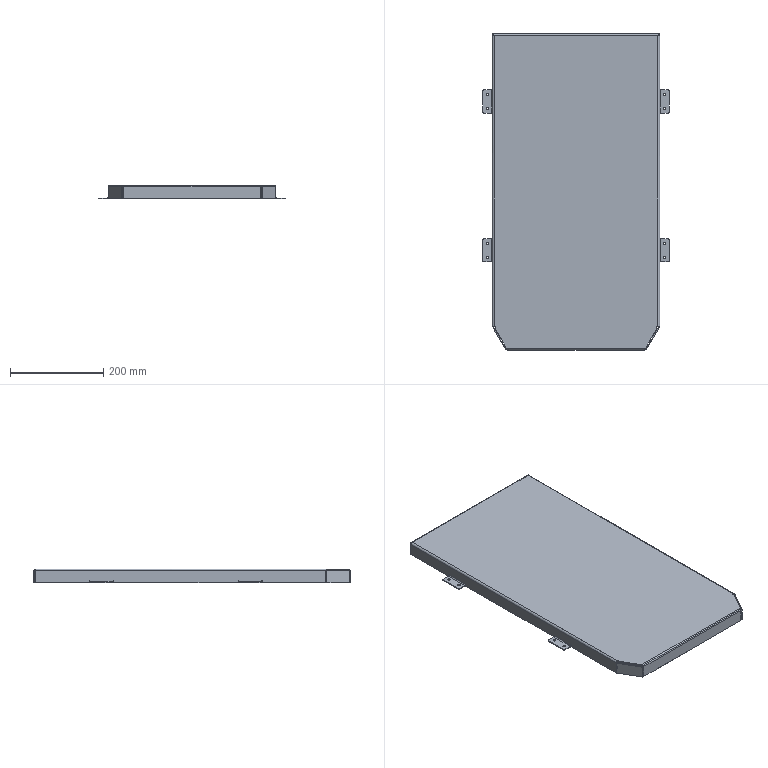Part | NX | features 5003_231_Plate 2 | 1 solid | 146 faces | box 400 x 679.316 x 30 mm | volume 600016 mm3 | plane 99 | cylinder 37 | spline 10 | commonest cylinder face diameters 4 x19 8 x10 5.5 x8